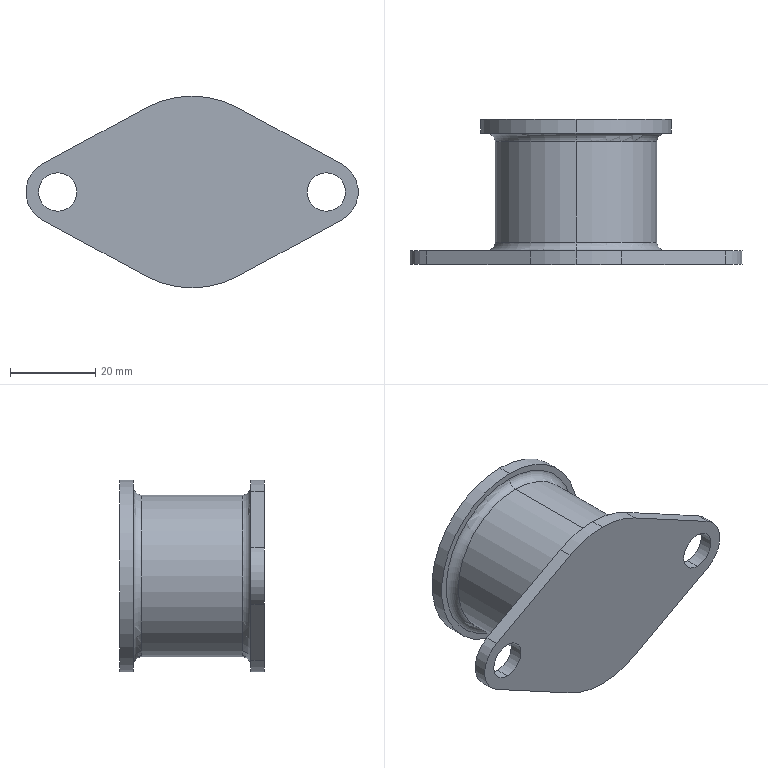Part | STEP file | SceondRB-45 | 1 solid | 29 faces | box 78 x 34 x 45 mm | volume 42765 mm3 | cylinder 15 | plane 8 | torus 4 | cone 2 | commonest cylinder face diameters 45 x5 9 x4 6.8 x2 15 x2 38 x2
STEP:
#1=CARTESIAN_POINT('',(0.,-19.75,-3.4));
#2=VERTEX_POINT('',#1);
#3=CARTESIAN_POINT('',(0.,-19.75,3.4));
#4=VERTEX_POINT('',#3);
#5=CARTESIAN_POINT('',(0.,-19.75,0.));
#6=DIRECTION('',(0.,1.,0.));
#7=DIRECTION('',(0.,0.,1.));
#8=AXIS2_PLACEMENT_3D('',#5,#6,#7);
#9=CIRCLE('',#8,3.4);
#10=EDGE_CURVE('',#2,#4,#9,.T.);
#11=ORIENTED_EDGE('',*,*,#10,.F.);
#12=CARTESIAN_POINT('',(0.,0.,-3.4));
#13=VERTEX_POINT('',#12);
#14=CARTESIAN_POINT('',(0.,0.,-3.4));
#15=DIRECTION('',(0.,1.,0.));
#16=VECTOR('',#15,1000.);
#17=LINE('',#14,#16);
#18=EDGE_CURVE('',#2,#13,#17,.T.);
#19=ORIENTED_EDGE('',*,*,#18,.T.);
#20=CARTESIAN_POINT('',(0.,0.,3.4));
#21=VERTEX_POINT('',#20);
#22=CARTESIAN_POINT('',(0.,0.,0.));
#23=DIRECTION('',(0.,1.,0.));
#24=DIRECTION('',(0.,0.,1.));
#25=AXIS2_PLACEMENT_3D('',#22,#23,#24);
#26=CIRCLE('',#25,3.4);
#27=EDGE_CURVE('',#13,#21,#26,.T.);
#28=ORIENTED_EDGE('',*,*,#27,.T.);
#29=CARTESIAN_POINT('',(0.,0.,3.4));
#30=DIRECTION('',(0.,1.,0.));
#31=VECTOR('',#30,1000.);
#32=LINE('',#29,#31);
#33=EDGE_CURVE('',#4,#21,#32,.T.);
#34=ORIENTED_EDGE('',*,*,#33,.F.);
#35=EDGE_LOOP('',(#11,#19,#28,#34));
#36=FACE_OUTER_BOUND('',#35,.T.);
#37=CARTESIAN_POINT('',(0.,0.,0.));
#38=DIRECTION('',(0.,1.,0.));
#39=DIRECTION('',(0.,0.,1.));
#40=AXIS2_PLACEMENT_3D('',#37,#38,#39);
#41=CYLINDRICAL_SURFACE('',#40,3.4);
#42=ADVANCED_FACE('',(#36),#41,.F.);
#43=CARTESIAN_POINT('',(0.,-21.793,0.));
#44=VERTEX_POINT('',#43);
#45=CARTESIAN_POINT('',(0.,-19.75,3.4));
#46=DIRECTION('',(0.,0.515,0.8572));
#47=VECTOR('',#46,1000.);
#48=LINE('',#45,#47);
#49=EDGE_CURVE('',#44,#4,#48,.T.);
#50=ORIENTED_EDGE('',*,*,#49,.F.);
#51=CARTESIAN_POINT('',(0.,-19.75,-3.4));
#52=DIRECTION('',(0.,0.515,-0.8572));
#53=VECTOR('',#52,1000.);
#54=LINE('',#51,#53);
#55=EDGE_CURVE('',#44,#2,#54,.T.);
#56=ORIENTED_EDGE('',*,*,#55,.T.);
#57=ORIENTED_EDGE('',*,*,#10,.T.);
#58=EDGE_LOOP('',(#50,#56,#57));
#59=FACE_OUTER_BOUND('',#58,.T.);
#60=CARTESIAN_POINT('',(0.,-19.75,0.));
#61=DIRECTION('',(0.,1.,0.));
#62=DIRECTION('',(0.,0.,1.));
#63=AXIS2_PLACEMENT_3D('',#60,#61,#62);
#64=CONICAL_SURFACE('',#63,3.4,1.03);
#65=ADVANCED_FACE('',(#59),#64,.F.);
#66=CARTESIAN_POINT('',(31.5,-34.,4.5));
#67=VERTEX_POINT('',#66);
#68=CARTESIAN_POINT('',(31.5,-34.,-4.5));
#69=VERTEX_POINT('',#68);
#70=CARTESIAN_POINT('',(31.5,-34.,0.));
#71=DIRECTION('',(0.,-1.,0.));
#72=DIRECTION('',(0.,0.,-1.));
#73=AXIS2_PLACEMENT_3D('',#70,#71,#72);
#74=CIRCLE('',#73,4.5);
#75=EDGE_CURVE('',#67,#69,#74,.T.);
#76=ORIENTED_EDGE('',*,*,#75,.T.);
#77=CARTESIAN_POINT('',(31.5,-30.8,-4.5));
#78=VERTEX_POINT('',#77);
#79=CARTESIAN_POINT('',(31.5,-34.,-4.5));
#80=DIRECTION('',(0.,1.,0.));
#81=VECTOR('',#80,1000.);
#82=LINE('',#79,#81);
#83=EDGE_CURVE('',#69,#78,#82,.T.);
#84=ORIENTED_EDGE('',*,*,#83,.T.);
#85=CARTESIAN_POINT('',(31.5,-30.8,4.5));
#86=VERTEX_POINT('',#85);
#87=CARTESIAN_POINT('',(31.5,-30.8,0.));
#88=DIRECTION('',(0.,-1.,0.));
#89=DIRECTION('',(0.,0.,-1.));
#90=AXIS2_PLACEMENT_3D('',#87,#88,#89);
#91=CIRCLE('',#90,4.5);
#92=EDGE_CURVE('',#86,#78,#91,.T.);
#93=ORIENTED_EDGE('',*,*,#92,.F.);
#94=CARTESIAN_POINT('',(31.5,-34.,4.5));
#95=DIRECTION('',(0.,1.,0.));
#96=VECTOR('',#95,1000.);
#97=LINE('',#94,#96);
#98=EDGE_CURVE('',#67,#86,#97,.T.);
#99=ORIENTED_EDGE('',*,*,#98,.F.);
#100=EDGE_LOOP('',(#76,#84,#93,#99));
#101=FACE_OUTER_BOUND('',#100,.T.);
#102=CARTESIAN_POINT('',(31.5,-34.,0.));
#103=DIRECTION('',(0.,1.,0.));
#104=DIRECTION('',(0.,0.,1.));
#105=AXIS2_PLACEMENT_3D('',#102,#103,#104);
#106=CYLINDRICAL_SURFACE('',#105,4.5);
#107=ADVANCED_FACE('',(#101),#106,.F.);
#108=CARTESIAN_POINT('',(-31.5,-34.,4.5));
#109=VERTEX_POINT('',#108);
#110=CARTESIAN_POINT('',(-31.5,-34.,-4.5));
#111=VERTEX_POINT('',#110);
#112=CARTESIAN_POINT('',(-31.5,-34.,0.));
#113=DIRECTION('',(0.,-1.,0.));
#114=DIRECTION('',(0.,0.,-1.));
#115=AXIS2_PLACEMENT_3D('',#112,#113,#114);
#116=CIRCLE('',#115,4.5);
#117=EDGE_CURVE('',#109,#111,#116,.T.);
#118=ORIENTED_EDGE('',*,*,#117,.T.);
#119=CARTESIAN_POINT('',(-31.5,-30.8,-4.5));
#120=VERTEX_POINT('',#119);
#121=CARTESIAN_POINT('',(-31.5,-34.,-4.5));
#122=DIRECTION('',(0.,1.,0.));
#123=VECTOR('',#122,1000.);
#124=LINE('',#121,#123);
#125=EDGE_CURVE('',#111,#120,#124,.T.);
#126=ORIENTED_EDGE('',*,*,#125,.T.);
#127=CARTESIAN_POINT('',(-31.5,-30.8,4.5));
#128=VERTEX_POINT('',#127);
#129=CARTESIAN_POINT('',(-31.5,-30.8,0.));
#130=DIRECTION('',(0.,-1.,0.));
#131=DIRECTION('',(0.,0.,-1.));
#132=AXIS2_PLACEMENT_3D('',#129,#130,#131);
#133=CIRCLE('',#132,4.5);
#134=EDGE_CURVE('',#128,#120,#133,.T.);
#135=ORIENTED_EDGE('',*,*,#134,.F.);
#136=CARTESIAN_POINT('',(-31.5,-34.,4.5));
#137=DIRECTION('',(0.,1.,0.));
#138=VECTOR('',#137,1000.);
#139=LINE('',#136,#138);
#140=EDGE_CURVE('',#109,#128,#139,.T.);
#141=ORIENTED_EDGE('',*,*,#140,.F.);
#142=EDGE_LOOP('',(#118,#126,#135,#141));
#143=FACE_OUTER_BOUND('',#142,.T.);
#144=CARTESIAN_POINT('',(-31.5,-34.,0.));
#145=DIRECTION('',(0.,1.,0.));
#146=DIRECTION('',(0.,0.,1.));
#147=AXIS2_PLACEMENT_3D('',#144,#145,#146);
#148=CYLINDRICAL_SURFACE('',#147,4.5);
#149=ADVANCED_FACE('',(#143),#148,.F.);
#150=CARTESIAN_POINT('',(0.,-34.,22.5));
#151=VERTEX_POINT('',#150);
#152=CARTESIAN_POINT('',(-10.714,-34.,19.785));
#153=VERTEX_POINT('',#152);
#154=CARTESIAN_POINT('',(0.,-34.,0.));
#155=DIRECTION('',(0.,-1.,0.));
#156=DIRECTION('',(0.,0.,-1.));
#157=AXIS2_PLACEMENT_3D('',#154,#155,#156);
#158=CIRCLE('',#157,22.5);
#159=EDGE_CURVE('',#151,#153,#158,.T.);
#160=ORIENTED_EDGE('',*,*,#159,.F.);
#161=CARTESIAN_POINT('',(0.,-30.8,22.5));
#162=VERTEX_POINT('',#161);
#163=CARTESIAN_POINT('',(0.,-34.,22.5));
#164=DIRECTION('',(0.,1.,0.));
#165=VECTOR('',#164,1000.);
#166=LINE('',#163,#165);
#167=EDGE_CURVE('',#151,#162,#166,.T.);
#168=ORIENTED_EDGE('',*,*,#167,.T.);
#169=CARTESIAN_POINT('',(-10.714,-30.8,19.785));
#170=VERTEX_POINT('',#169);
#171=CARTESIAN_POINT('',(0.,-30.8,0.));
#172=DIRECTION('',(0.,-1.,0.));
#173=DIRECTION('',(0.,0.,-1.));
#174=AXIS2_PLACEMENT_3D('',#171,#172,#173);
#175=CIRCLE('',#174,22.5);
#176=EDGE_CURVE('',#162,#170,#175,.T.);
#177=ORIENTED_EDGE('',*,*,#176,.T.);
#178=CARTESIAN_POINT('',(-10.714,-34.,19.785));
#179=DIRECTION('',(0.,1.,0.));
#180=VECTOR('',#179,1000.);
#181=LINE('',#178,#180);
#182=EDGE_CURVE('',#153,#170,#181,.T.);
#183=ORIENTED_EDGE('',*,*,#182,.F.);
#184=EDGE_LOOP('',(#160,#168,#177,#183));
#185=FACE_OUTER_BOUND('',#184,.T.);
#186=CARTESIAN_POINT('',(0.,-34.,0.));
#187=DIRECTION('',(0.,1.,0.));
#188=DIRECTION('',(0.,0.,1.));
#189=AXIS2_PLACEMENT_3D('',#186,#187,#188);
#190=CYLINDRICAL_SURFACE('',#189,22.5);
#191=ADVANCED_FACE('',(#185),#190,.T.);
#192=CARTESIAN_POINT('',(0.,-3.2,-21.));
#193=VERTEX_POINT('',#192);
#194=CARTESIAN_POINT('',(0.,-3.2,21.));
#195=VERTEX_POINT('',#194);
#196=CARTESIAN_POINT('',(0.,-3.2,0.));
#197=DIRECTION('',(0.,1.,0.));
#198=DIRECTION('',(0.,0.,1.));
#199=AXIS2_PLACEMENT_3D('',#196,#197,#198);
#200=CIRCLE('',#199,21.);
#201=EDGE_CURVE('',#193,#195,#200,.T.);
#202=ORIENTED_EDGE('',*,*,#201,.F.);
#203=CARTESIAN_POINT('',(0.,-5.2,-19.));
#204=VERTEX_POINT('',#203);
#205=CARTESIAN_POINT('',(0.,-5.2,-21.));
#206=DIRECTION('',(1.,0.,0.));
#207=DIRECTION('',(0.,0.,-1.));
#208=AXIS2_PLACEMENT_3D('',#205,#206,#207);
#209=CIRCLE('',#208,2.);
#210=EDGE_CURVE('',#193,#204,#209,.T.);
#211=ORIENTED_EDGE('',*,*,#210,.T.);
#212=CARTESIAN_POINT('',(0.,-5.2,19.));
#213=VERTEX_POINT('',#212);
#214=CARTESIAN_POINT('',(0.,-5.2,0.));
#215=DIRECTION('',(0.,1.,0.));
#216=DIRECTION('',(0.,0.,1.));
#217=AXIS2_PLACEMENT_3D('',#214,#215,#216);
#218=CIRCLE('',#217,19.);
#219=EDGE_CURVE('',#204,#213,#218,.T.);
#220=ORIENTED_EDGE('',*,*,#219,.T.);
#221=CARTESIAN_POINT('',(0.,-5.2,21.));
#222=DIRECTION('',(-1.,0.,0.));
#223=DIRECTION('',(0.,0.,1.));
#224=AXIS2_PLACEMENT_3D('',#221,#222,#223);
#225=CIRCLE('',#224,2.);
#226=EDGE_CURVE('',#195,#213,#225,.T.);
#227=ORIENTED_EDGE('',*,*,#226,.F.);
#228=EDGE_LOOP('',(#202,#211,#220,#227));
#229=FACE_OUTER_BOUND('',#228,.T.);
#230=CARTESIAN_POINT('',(0.,-5.2,0.));
#231=DIRECTION('',(0.,1.,0.));
#232=DIRECTION('',(0.,0.,1.));
#233=AXIS2_PLACEMENT_3D('',#230,#231,#232);
#234=TOROIDAL_SURFACE('',#233,21.,2.);
#235=ADVANCED_FACE('',(#229),#234,.F.);
#236=CARTESIAN_POINT('',(0.,-28.8,19.));
#237=VERTEX_POINT('',#236);
#238=CARTESIAN_POINT('',(0.,-28.8,-19.));
#239=VERTEX_POINT('',#238);
#240=CARTESIAN_POINT('',(0.,-28.8,0.));
#241=DIRECTION('',(0.,1.,0.));
#242=DIRECTION('',(0.,0.,1.));
#243=AXIS2_PLACEMENT_3D('',#240,#241,#242);
#244=CIRCLE('',#243,19.);
#245=EDGE_CURVE('',#237,#239,#244,.T.);
#246=ORIENTED_EDGE('',*,*,#245,.T.);
#247=CARTESIAN_POINT('',(0.,0.,-19.));
#248=DIRECTION('',(0.,1.,0.));
#249=VECTOR('',#248,1000.);
#250=LINE('',#247,#249);
#251=EDGE_CURVE('',#239,#204,#250,.T.);
#252=ORIENTED_EDGE('',*,*,#251,.T.);
#253=CARTESIAN_POINT('',(0.,-5.2,0.));
#254=DIRECTION('',(0.,1.,0.));
#255=DIRECTION('',(0.,0.,1.));
#256=AXIS2_PLACEMENT_3D('',#253,#254,#255);
#257=CIRCLE('',#256,19.);
#258=EDGE_CURVE('',#213,#204,#257,.T.);
#259=ORIENTED_EDGE('',*,*,#258,.F.);
#260=CARTESIAN_POINT('',(0.,0.,19.));
#261=DIRECTION('',(0.,1.,0.));
#262=VECTOR('',#261,1000.);
#263=LINE('',#260,#262);
#264=EDGE_CURVE('',#237,#213,#263,.T.);
#265=ORIENTED_EDGE('',*,*,#264,.F.);
#266=EDGE_LOOP('',(#246,#252,#259,#265));
#267=FACE_OUTER_BOUND('',#266,.T.);
#268=CARTESIAN_POINT('',(0.,0.,0.));
#269=DIRECTION('',(0.,1.,0.));
#270=DIRECTION('',(0.,0.,1.));
#271=AXIS2_PLACEMENT_3D('',#268,#269,#270);
#272=CYLINDRICAL_SURFACE('',#271,19.);
#273=ADVANCED_FACE('',(#267),#272,.T.);
#274=CARTESIAN_POINT('',(0.,-28.8,0.));
#275=DIRECTION('',(0.,1.,0.));
#276=DIRECTION('',(0.,0.,1.));
#277=AXIS2_PLACEMENT_3D('',#274,#275,#276);
#278=CIRCLE('',#277,19.);
#279=EDGE_CURVE('',#239,#237,#278,.T.);
#280=ORIENTED_EDGE('',*,*,#279,.F.);
#281=CARTESIAN_POINT('',(0.,-30.8,-21.));
#282=VERTEX_POINT('',#281);
#283=CARTESIAN_POINT('',(0.,-28.8,-21.));
#284=DIRECTION('',(1.,0.,0.));
#285=DIRECTION('',(0.,0.,-1.));
#286=AXIS2_PLACEMENT_3D('',#283,#284,#285);
#287=CIRCLE('',#286,2.);
#288=EDGE_CURVE('',#239,#282,#287,.T.);
#289=ORIENTED_EDGE('',*,*,#288,.T.);
#290=CARTESIAN_POINT('',(0.,-30.8,21.));
#291=VERTEX_POINT('',#290);
#292=CARTESIAN_POINT('',(0.,-30.8,0.));
#293=DIRECTION('',(0.,-1.,0.));
#294=DIRECTION('',(0.,0.,1.));
#295=AXIS2_PLACEMENT_3D('',#292,#293,#294);
#296=CIRCLE('',#295,21.);
#297=EDGE_CURVE('',#291,#282,#296,.T.);
#298=ORIENTED_EDGE('',*,*,#297,.F.);
#299=CARTESIAN_POINT('',(0.,-28.8,21.));
#300=DIRECTION('',(-1.,0.,0.));
#301=DIRECTION('',(0.,0.,1.));
#302=AXIS2_PLACEMENT_3D('',#299,#300,#301);
#303=CIRCLE('',#302,2.);
#304=EDGE_CURVE('',#237,#291,#303,.T.);
#305=ORIENTED_EDGE('',*,*,#304,.F.);
#306=EDGE_LOOP('',(#280,#289,#298,#305));
#307=FACE_OUTER_BOUND('',#306,.T.);
#308=CARTESIAN_POINT('',(0.,-28.8,0.));
#309=DIRECTION('',(0.,1.,0.));
#310=DIRECTION('',(0.,0.,1.));
#311=AXIS2_PLACEMENT_3D('',#308,#309,#310);
#312=TOROIDAL_SURFACE('',#311,21.,2.);
#313=ADVANCED_FACE('',(#307),#312,.F.);
#314=CARTESIAN_POINT('',(0.,-3.2,22.5));
#315=VERTEX_POINT('',#314);
#316=CARTESIAN_POINT('',(0.,-3.2,-22.5));
#317=VERTEX_POINT('',#316);
#318=CARTESIAN_POINT('',(0.,-3.2,0.));
#319=DIRECTION('',(0.,1.,0.));
#320=DIRECTION('',(0.,0.,1.));
#321=AXIS2_PLACEMENT_3D('',#318,#319,#320);
#322=CIRCLE('',#321,22.5);
#323=EDGE_CURVE('',#315,#317,#322,.T.);
#324=ORIENTED_EDGE('',*,*,#323,.T.);
#325=CARTESIAN_POINT('',(0.,0.,-22.5));
#326=VERTEX_POINT('',#325);
#327=CARTESIAN_POINT('',(0.,0.,-22.5));
#328=DIRECTION('',(0.,1.,0.));
#329=VECTOR('',#328,1000.);
#330=LINE('',#327,#329);
#331=EDGE_CURVE('',#317,#326,#330,.T.);
#332=ORIENTED_EDGE('',*,*,#331,.T.);
#333=CARTESIAN_POINT('',(0.,0.,22.5));
#334=VERTEX_POINT('',#333);
#335=CARTESIAN_POINT('',(0.,0.,0.));
#336=DIRECTION('',(0.,1.,0.));
#337=DIRECTION('',(0.,0.,1.));
#338=AXIS2_PLACEMENT_3D('',#335,#336,#337);
#339=CIRCLE('',#338,22.5);
#340=EDGE_CURVE('',#334,#326,#339,.T.);
#341=ORIENTED_EDGE('',*,*,#340,.F.);
#342=CARTESIAN_POINT('',(0.,0.,22.5));
#343=DIRECTION('',(0.,1.,0.));
#344=VECTOR('',#343,1000.);
#345=LINE('',#342,#344);
#346=EDGE_CURVE('',#315,#334,#345,.T.);
#347=ORIENTED_EDGE('',*,*,#346,.F.);
#348=EDGE_LOOP('',(#324,#332,#341,#347));
#349=FACE_OUTER_BOUND('',#348,.T.);
#350=CARTESIAN_POINT('',(0.,0.,0.));
#351=DIRECTION('',(0.,1.,0.));
#352=DIRECTION('',(0.,0.,1.));
#353=AXIS2_PLACEMENT_3D('',#350,#351,#352);
#354=CYLINDRICAL_SURFACE('',#353,22.5);
#355=ADVANCED_FACE('',(#349),#354,.T.);
#356=ORIENTED_EDGE('',*,*,#331,.F.);
#357=CARTESIAN_POINT('',(0.,-3.2,0.));
#358=DIRECTION('',(0.,1.,0.));
#359=DIRECTION('',(0.,0.,1.));
#360=AXIS2_PLACEMENT_3D('',#357,#358,#359);
#361=CIRCLE('',#360,22.5);
#362=EDGE_CURVE('',#317,#315,#361,.T.);
#363=ORIENTED_EDGE('',*,*,#362,.T.);
#364=ORIENTED_EDGE('',*,*,#346,.T.);
#365=CARTESIAN_POINT('',(0.,0.,0.));
#366=DIRECTION('',(0.,1.,0.));
#367=DIRECTION('',(0.,0.,1.));
#368=AXIS2_PLACEMENT_3D('',#365,#366,#367);
#369=CIRCLE('',#368,22.5);
#370=EDGE_CURVE('',#326,#334,#369,.T.);
#371=ORIENTED_EDGE('',*,*,#370,.F.);
#372=EDGE_LOOP('',(#356,#363,#364,#371));
#373=FACE_OUTER_BOUND('',#372,.T.);
#374=CARTESIAN_POINT('',(0.,0.,0.));
#375=DIRECTION('',(0.,1.,0.));
#376=DIRECTION('',(0.,0.,1.));
#377=AXIS2_PLACEMENT_3D('',#374,#375,#376);
#378=CYLINDRICAL_SURFACE('',#377,22.5);
#379=ADVANCED_FACE('',(#373),#378,.T.);
#380=CARTESIAN_POINT('',(0.,0.,0.));
#381=DIRECTION('',(0.,1.,0.));
#382=DIRECTION('',(0.,0.,1.));
#383=AXIS2_PLACEMENT_3D('',#380,#381,#382);
#384=CIRCLE('',#383,3.4);
#385=EDGE_CURVE('',#21,#13,#384,.T.);
#386=ORIENTED_EDGE('',*,*,#385,.F.);
#387=ORIENTED_EDGE('',*,*,#27,.F.);
#388=EDGE_LOOP('',(#386,#387));
#389=FACE_BOUND('',#388,.T.);
#390=ORIENTED_EDGE('',*,*,#340,.T.);
#391=ORIENTED_EDGE('',*,*,#370,.T.);
#392=EDGE_LOOP('',(#390,#391));
#393=FACE_OUTER_BOUND('',#392,.T.);
#394=CARTESIAN_POINT('',(22.5,0.,0.));
#395=DIRECTION('',(0.,-1.,0.));
#396=DIRECTION('',(0.,0.,-1.));
#397=AXIS2_PLACEMENT_3D('',#394,#395,#396);
#398=PLANE('',#397);
#399=ADVANCED_FACE('',(#389,#393),#398,.F.);
#400=ORIENTED_EDGE('',*,*,#288,.F.);
#401=ORIENTED_EDGE('',*,*,#245,.F.);
#402=ORIENTED_EDGE('',*,*,#304,.T.);
#403=CARTESIAN_POINT('',(0.,-30.8,0.));
#404=DIRECTION('',(0.,-1.,0.));
#405=DIRECTION('',(0.,0.,1.));
#406=AXIS2_PLACEMENT_3D('',#403,#404,#405);
#407=CIRCLE('',#406,21.);
#408=EDGE_CURVE('',#282,#291,#407,.T.);
#409=ORIENTED_EDGE('',*,*,#408,.F.);
#410=EDGE_LOOP('',(#400,#401,#402,#409));
#411=FACE_OUTER_BOUND('',#410,.T.);
#412=CARTESIAN_POINT('',(0.,-28.8,0.));
#413=DIRECTION('',(0.,1.,0.));
#414=DIRECTION('',(0.,0.,1.));
#415=AXIS2_PLACEMENT_3D('',#412,#413,#414);
#416=TOROIDAL_SURFACE('',#415,21.,2.);
#417=ADVANCED_FACE('',(#411),#416,.F.);
#418=ORIENTED_EDGE('',*,*,#251,.F.);
#419=ORIENTED_EDGE('',*,*,#279,.T.);
#420=ORIENTED_EDGE('',*,*,#264,.T.);
#421=ORIENTED_EDGE('',*,*,#219,.F.);
#422=EDGE_LOOP('',(#418,#419,#420,#421));
#423=FACE_OUTER_BOUND('',#422,.T.);
#424=CARTESIAN_POINT('',(0.,0.,0.));
#425=DIRECTION('',(0.,1.,0.));
#426=DIRECTION('',(0.,0.,1.));
#427=AXIS2_PLACEMENT_3D('',#424,#425,#426);
#428=CYLINDRICAL_SURFACE('',#427,19.);
#429=ADVANCED_FACE('',(#423),#428,.T.);
#430=ORIENTED_EDGE('',*,*,#210,.F.);
#431=CARTESIAN_POINT('',(0.,-3.2,0.));
#432=DIRECTION('',(0.,1.,0.));
#433=DIRECTION('',(0.,0.,1.));
#434=AXIS2_PLACEMENT_3D('',#431,#432,#433);
#435=CIRCLE('',#434,21.);
#436=EDGE_CURVE('',#195,#193,#435,.T.);
#437=ORIENTED_EDGE('',*,*,#436,.F.);
#438=ORIENTED_EDGE('',*,*,#226,.T.);
#439=ORIENTED_EDGE('',*,*,#258,.T.);
#440=EDGE_LOOP('',(#430,#437,#438,#439));
#441=FACE_OUTER_BOUND('',#440,.T.);
#442=CARTESIAN_POINT('',(0.,-5.2,0.));
#443=DIRECTION('',(0.,1.,0.));
#444=DIRECTION('',(0.,0.,1.));
#445=AXIS2_PLACEMENT_3D('',#442,#443,#444);
#446=TOROIDAL_SURFACE('',#445,21.,2.);
#447=ADVANCED_FACE('',(#441),#446,.F.);
#448=ORIENTED_EDGE('',*,*,#323,.F.);
#449=ORIENTED_EDGE('',*,*,#362,.F.);
#450=EDGE_LOOP('',(#448,#449));
#451=FACE_OUTER_BOUND('',#450,.T.);
#452=ORIENTED_EDGE('',*,*,#436,.T.);
#453=ORIENTED_EDGE('',*,*,#201,.T.);
#454=EDGE_LOOP('',(#452,#453));
#455=FACE_BOUND('',#454,.T.);
#456=CARTESIAN_POINT('',(21.,-3.2,0.));
#457=DIRECTION('',(0.,1.,0.));
#458=DIRECTION('',(0.,0.,1.));
#459=AXIS2_PLACEMENT_3D('',#456,#457,#458);
#460=PLANE('',#459);
#461=ADVANCED_FACE('',(#451,#455),#460,.F.);
#462=ORIENTED_EDGE('',*,*,#92,.T.);
#463=CARTESIAN_POINT('',(31.5,-30.8,0.));
#464=DIRECTION('',(0.,-1.,0.));
#465=DIRECTION('',(0.,0.,-1.));
#466=AXIS2_PLACEMENT_3D('',#463,#464,#465);
#467=CIRCLE('',#466,4.5);
#468=EDGE_CURVE('',#78,#86,#467,.T.);
#469=ORIENTED_EDGE('',*,*,#468,.T.);
#470=EDGE_LOOP('',(#462,#469));
#471=FACE_BOUND('',#470,.T.);
#472=CARTESIAN_POINT('',(-35.071,-30.8,6.595));
#473=VERTEX_POINT('',#472);
#474=CARTESIAN_POINT('',(-35.071,-30.8,-6.595));
#475=VERTEX_POINT('',#474);
#476=CARTESIAN_POINT('',(-31.5,-30.8,0.));
#477=DIRECTION('',(0.,-1.,0.));
#478=DIRECTION('',(0.,0.,-1.));
#479=AXIS2_PLACEMENT_3D('',#476,#477,#478);
#480=CIRCLE('',#479,7.5);
#481=EDGE_CURVE('',#473,#475,#480,.T.);
#482=ORIENTED_EDGE('',*,*,#481,.F.);
#483=CARTESIAN_POINT('',(-35.071,-30.8,6.595));
#484=DIRECTION('',(-0.8793,0.,-0.4762));
#485=VECTOR('',#484,1000.);
#486=LINE('',#483,#485);
#487=EDGE_CURVE('',#170,#473,#486,.T.);
#488=ORIENTED_EDGE('',*,*,#487,.F.);
#489=ORIENTED_EDGE('',*,*,#176,.F.);
#490=CARTESIAN_POINT('',(10.714,-30.8,19.785));
#491=VERTEX_POINT('',#490);
#492=CARTESIAN_POINT('',(0.,-30.8,0.));
#493=DIRECTION('',(0.,-1.,0.));
#494=DIRECTION('',(0.,0.,-1.));
#495=AXIS2_PLACEMENT_3D('',#492,#493,#494);
#496=CIRCLE('',#495,22.5);
#497=EDGE_CURVE('',#491,#162,#496,.T.);
#498=ORIENTED_EDGE('',*,*,#497,.F.);
#499=CARTESIAN_POINT('',(35.071,-30.8,6.595));
#500=VERTEX_POINT('',#499);
#501=CARTESIAN_POINT('',(10.714,-30.8,19.785));
#502=DIRECTION('',(-0.8793,0.,0.4762));
#503=VECTOR('',#502,1000.);
#504=LINE('',#501,#503);
#505=EDGE_CURVE('',#500,#491,#504,.T.);
#506=ORIENTED_EDGE('',*,*,#505,.F.);
#507=CARTESIAN_POINT('',(35.071,-30.8,-6.595));
#508=VERTEX_POINT('',#507);
#509=CARTESIAN_POINT('',(31.5,-30.8,0.));
#510=DIRECTION('',(0.,-1.,0.));
#511=DIRECTION('',(0.,0.,-1.));
#512=AXIS2_PLACEMENT_3D('',#509,#510,#511);
#513=CIRCLE('',#512,7.5);
#514=EDGE_CURVE('',#508,#500,#513,.T.);
#515=ORIENTED_EDGE('',*,*,#514,.F.);
#516=CARTESIAN_POINT('',(10.714,-30.8,-19.785));
#517=VERTEX_POINT('',#516);
#518=CARTESIAN_POINT('',(10.714,-30.8,-19.785));
#519=DIRECTION('',(0.8793,0.,0.4762));
#520=VECTOR('',#519,1000.);
#521=LINE('',#518,#520);
#522=EDGE_CURVE('',#517,#508,#521,.T.);
#523=ORIENTED_EDGE('',*,*,#522,.F.);
#524=CARTESIAN_POINT('',(-10.714,-30.8,-19.785));
#525=VERTEX_POINT('',#524);
#526=CARTESIAN_POINT('',(0.,-30.8,0.));
#527=DIRECTION('',(0.,-1.,0.));
#528=DIRECTION('',(0.,0.,-1.));
#529=AXIS2_PLACEMENT_3D('',#526,#527,#528);
#530=CIRCLE('',#529,22.5);
#531=EDGE_CURVE('',#525,#517,#530,.T.);
#532=ORIENTED_EDGE('',*,*,#531,.F.);
#533=CARTESIAN_POINT('',(-35.071,-30.8,-6.595));
#534=DIRECTION('',(0.8793,0.,-0.4762));
#535=VECTOR('',#534,1000.);
#536=LINE('',#533,#535);
#537=EDGE_CURVE('',#475,#525,#536,.T.);
#538=ORIENTED_EDGE('',*,*,#537,.F.);
#539=EDGE_LOOP('',(#482,#488,#489,#498,#506,#515,#523,#532,#538));
#540=FACE_OUTER_BOUND('',#539,.T.);
#541=ORIENTED_EDGE('',*,*,#134,.T.);
#542=CARTESIAN_POINT('',(-31.5,-30.8,0.));
#543=DIRECTION('',(0.,-1.,0.));
#544=DIRECTION('',(0.,0.,-1.));
#545=AXIS2_PLACEMENT_3D('',#542,#543,#544);
#546=CIRCLE('',#545,4.5);
#547=EDGE_CURVE('',#120,#128,#546,.T.);
#548=ORIENTED_EDGE('',*,*,#547,.T.);
#549=EDGE_LOOP('',(#541,#548));
#550=FACE_BOUND('',#549,.T.);
#551=ORIENTED_EDGE('',*,*,#297,.T.);
#552=ORIENTED_EDGE('',*,*,#408,.T.);
#553=EDGE_LOOP('',(#551,#552));
#554=FACE_BOUND('',#553,.T.);
#555=CARTESIAN_POINT('',(-31.5,-30.8,0.));
#556=DIRECTION('',(0.,-1.,0.));
#557=DIRECTION('',(0.,0.,-1.));
#558=AXIS2_PLACEMENT_3D('',#555,#556,#557);
#559=PLANE('',#558);
#560=ADVANCED_FACE('',(#471,#540,#550,#554),#559,.F.);
#561=ORIENTED_EDGE('',*,*,#117,.F.);
#562=CARTESIAN_POINT('',(-31.5,-34.,0.));
#563=DIRECTION('',(0.,-1.,0.));
#564=DIRECTION('',(0.,0.,-1.));
#565=AXIS2_PLACEMENT_3D('',#562,#563,#564);
#566=CIRCLE('',#565,4.5);
#567=EDGE_CURVE('',#111,#109,#566,.T.);
#568=ORIENTED_EDGE('',*,*,#567,.F.);
#569=EDGE_LOOP('',(#561,#568));
#570=FACE_BOUND('',#569,.T.);
#571=CARTESIAN_POINT('',(-35.071,-34.,6.595));
#572=VERTEX_POINT('',#571);
#573=CARTESIAN_POINT('',(-35.071,-34.,-6.595));
#574=VERTEX_POINT('',#573);
#575=CARTESIAN_POINT('',(-31.5,-34.,0.));
#576=DIRECTION('',(0.,-1.,0.));
#577=DIRECTION('',(0.,0.,-1.));
#578=AXIS2_PLACEMENT_3D('',#575,#576,#577);
#579=CIRCLE('',#578,7.5);
#580=EDGE_CURVE('',#572,#574,#579,.T.);
#581=ORIENTED_EDGE('',*,*,#580,.T.);
#582=CARTESIAN_POINT('',(-10.714,-34.,-19.785));
#583=VERTEX_POINT('',#582);
#584=CARTESIAN_POINT('',(-35.071,-34.,-6.595));
#585=DIRECTION('',(0.8793,0.,-0.4762));
#586=VECTOR('',#585,1000.);
#587=LINE('',#584,#586);
#588=EDGE_CURVE('',#574,#583,#587,.T.);
#589=ORIENTED_EDGE('',*,*,#588,.T.);
#590=CARTESIAN_POINT('',(10.714,-34.,-19.785));
#591=VERTEX_POINT('',#590);
#592=CARTESIAN_POINT('',(0.,-34.,0.));
#593=DIRECTION('',(0.,-1.,0.));
#594=DIRECTION('',(0.,0.,-1.));
#595=AXIS2_PLACEMENT_3D('',#592,#593,#594);
#596=CIRCLE('',#595,22.5);
#597=EDGE_CURVE('',#583,#591,#596,.T.);
#598=ORIENTED_EDGE('',*,*,#597,.T.);
#599=CARTESIAN_POINT('',(35.071,-34.,-6.595));
#600=VERTEX_POINT('',#599);
#601=CARTESIAN_POINT('',(10.714,-34.,-19.785));
#602=DIRECTION('',(0.8793,0.,0.4762));
#603=VECTOR('',#602,1000.);
#604=LINE('',#601,#603);
#605=EDGE_CURVE('',#591,#600,#604,.T.);
#606=ORIENTED_EDGE('',*,*,#605,.T.);
#607=CARTESIAN_POINT('',(35.071,-34.,6.595));
#608=VERTEX_POINT('',#607);
#609=CARTESIAN_POINT('',(31.5,-34.,0.));
#610=DIRECTION('',(0.,-1.,0.));
#611=DIRECTION('',(0.,0.,-1.));
#612=AXIS2_PLACEMENT_3D('',#609,#610,#611);
#613=CIRCLE('',#612,7.5);
#614=EDGE_CURVE('',#600,#608,#613,.T.);
#615=ORIENTED_EDGE('',*,*,#614,.T.);
#616=CARTESIAN_POINT('',(10.714,-34.,19.785));
#617=VERTEX_POINT('',#616);
#618=CARTESIAN_POINT('',(10.714,-34.,19.785));
#619=DIRECTION('',(-0.8793,0.,0.4762));
#620=VECTOR('',#619,1000.);
#621=LINE('',#618,#620);
#622=EDGE_CURVE('',#608,#617,#621,.T.);
#623=ORIENTED_EDGE('',*,*,#622,.T.);
#624=CARTESIAN_POINT('',(0.,-34.,0.));
#625=DIRECTION('',(0.,-1.,0.));
#626=DIRECTION('',(0.,0.,-1.));
#627=AXIS2_PLACEMENT_3D('',#624,#625,#626);
#628=CIRCLE('',#627,22.5);
#629=EDGE_CURVE('',#617,#151,#628,.T.);
#630=ORIENTED_EDGE('',*,*,#629,.T.);
#631=ORIENTED_EDGE('',*,*,#159,.T.);
#632=CARTESIAN_POINT('',(-35.071,-34.,6.595));
#633=DIRECTION('',(-0.8793,0.,-0.4762));
#634=VECTOR('',#633,1000.);
#635=LINE('',#632,#634);
#636=EDGE_CURVE('',#153,#572,#635,.T.);
#637=ORIENTED_EDGE('',*,*,#636,.T.);
#638=EDGE_LOOP('',(#581,#589,#598,#606,#615,#623,#630,#631,#637));
#639=FACE_OUTER_BOUND('',#638,.T.);
#640=ORIENTED_EDGE('',*,*,#75,.F.);
#641=CARTESIAN_POINT('',(31.5,-34.,0.));
#642=DIRECTION('',(0.,-1.,0.));
#643=DIRECTION('',(0.,0.,-1.));
#644=AXIS2_PLACEMENT_3D('',#641,#642,#643);
#645=CIRCLE('',#644,4.5);
#646=EDGE_CURVE('',#69,#67,#645,.T.);
#647=ORIENTED_EDGE('',*,*,#646,.F.);
#648=EDGE_LOOP('',(#640,#647));
#649=FACE_BOUND('',#648,.T.);
#650=CARTESIAN_POINT('',(-31.5,-34.,0.));
#651=DIRECTION('',(0.,-1.,0.));
#652=DIRECTION('',(0.,0.,-1.));
#653=AXIS2_PLACEMENT_3D('',#650,#651,#652);
#654=PLANE('',#653);
#655=ADVANCED_FACE('',(#570,#639,#649),#654,.T.);
#656=ORIENTED_EDGE('',*,*,#481,.T.);
#657=CARTESIAN_POINT('',(-35.071,-34.,-6.595));
#658=DIRECTION('',(0.,1.,0.));
#659=VECTOR('',#658,1000.);
#660=LINE('',#657,#659);
#661=EDGE_CURVE('',#574,#475,#660,.T.);
#662=ORIENTED_EDGE('',*,*,#661,.F.);
#663=ORIENTED_EDGE('',*,*,#580,.F.);
#664=CARTESIAN_POINT('',(-35.071,-34.,6.595));
#665=DIRECTION('',(0.,1.,0.));
#666=VECTOR('',#665,1000.);
#667=LINE('',#664,#666);
#668=EDGE_CURVE('',#572,#473,#667,.T.);
#669=ORIENTED_EDGE('',*,*,#668,.T.);
#670=EDGE_LOOP('',(#656,#662,#663,#669));
#671=FACE_OUTER_BOUND('',#670,.T.);
#672=CARTESIAN_POINT('',(-31.5,-34.,0.));
#673=DIRECTION('',(0.,1.,0.));
#674=DIRECTION('',(0.,0.,1.));
#675=AXIS2_PLACEMENT_3D('',#672,#673,#674);
#676=CYLINDRICAL_SURFACE('',#675,7.5);
#677=ADVANCED_FACE('',(#671),#676,.T.);
#678=ORIENTED_EDGE('',*,*,#537,.T.);
#679=CARTESIAN_POINT('',(-10.714,-34.,-19.785));
#680=DIRECTION('',(0.,1.,0.));
#681=VECTOR('',#680,1000.);
#682=LINE('',#679,#681);
#683=EDGE_CURVE('',#583,#525,#682,.T.);
#684=ORIENTED_EDGE('',*,*,#683,.F.);
#685=ORIENTED_EDGE('',*,*,#588,.F.);
#686=ORIENTED_EDGE('',*,*,#661,.T.);
#687=EDGE_LOOP('',(#678,#684,#685,#686));
#688=FACE_OUTER_BOUND('',#687,.T.);
#689=CARTESIAN_POINT('',(-35.071,-34.,-6.595));
#690=DIRECTION('',(0.4762,0.,0.8793));
#691=DIRECTION('',(0.8793,0.,-0.4762));
#692=AXIS2_PLACEMENT_3D('',#689,#690,#691);
#693=PLANE('',#692);
#694=ADVANCED_FACE('',(#688),#693,.F.);
#695=ORIENTED_EDGE('',*,*,#531,.T.);
#696=CARTESIAN_POINT('',(10.714,-34.,-19.785));
#697=DIRECTION('',(0.,1.,0.));
#698=VECTOR('',#697,1000.);
#699=LINE('',#696,#698);
#700=EDGE_CURVE('',#591,#517,#699,.T.);
#701=ORIENTED_EDGE('',*,*,#700,.F.);
#702=ORIENTED_EDGE('',*,*,#597,.F.);
#703=ORIENTED_EDGE('',*,*,#683,.T.);
#704=EDGE_LOOP('',(#695,#701,#702,#703));
#705=FACE_OUTER_BOUND('',#704,.T.);
#706=CARTESIAN_POINT('',(0.,-34.,0.));
#707=DIRECTION('',(0.,1.,0.));
#708=DIRECTION('',(0.,0.,1.));
#709=AXIS2_PLACEMENT_3D('',#706,#707,#708);
#710=CYLINDRICAL_SURFACE('',#709,22.5);
#711=ADVANCED_FACE('',(#705),#710,.T.);
#712=ORIENTED_EDGE('',*,*,#522,.T.);
#713=CARTESIAN_POINT('',(35.071,-34.,-6.595));
#714=DIRECTION('',(0.,1.,0.));
#715=VECTOR('',#714,1000.);
#716=LINE('',#713,#715);
#717=EDGE_CURVE('',#600,#508,#716,.T.);
#718=ORIENTED_EDGE('',*,*,#717,.F.);
#719=ORIENTED_EDGE('',*,*,#605,.F.);
#720=ORIENTED_EDGE('',*,*,#700,.T.);
#721=EDGE_LOOP('',(#712,#718,#719,#720));
#722=FACE_OUTER_BOUND('',#721,.T.);
#723=CARTESIAN_POINT('',(10.714,-34.,-19.785));
#724=DIRECTION('',(-0.4762,0.,0.8793));
#725=DIRECTION('',(0.8793,0.,0.4762));
#726=AXIS2_PLACEMENT_3D('',#723,#724,#725);
#727=PLANE('',#726);
#728=ADVANCED_FACE('',(#722),#727,.F.);
#729=ORIENTED_EDGE('',*,*,#514,.T.);
#730=CARTESIAN_POINT('',(35.071,-34.,6.595));
#731=DIRECTION('',(0.,1.,0.));
#732=VECTOR('',#731,1000.);
#733=LINE('',#730,#732);
#734=EDGE_CURVE('',#608,#500,#733,.T.);
#735=ORIENTED_EDGE('',*,*,#734,.F.);
#736=ORIENTED_EDGE('',*,*,#614,.F.);
#737=ORIENTED_EDGE('',*,*,#717,.T.);
#738=EDGE_LOOP('',(#729,#735,#736,#737));
#739=FACE_OUTER_BOUND('',#738,.T.);
#740=CARTESIAN_POINT('',(31.5,-34.,0.));
#741=DIRECTION('',(0.,1.,0.));
#742=DIRECTION('',(0.,0.,1.));
#743=AXIS2_PLACEMENT_3D('',#740,#741,#742);
#744=CYLINDRICAL_SURFACE('',#743,7.5);
#745=ADVANCED_FACE('',(#739),#744,.T.);
#746=ORIENTED_EDGE('',*,*,#505,.T.);
#747=CARTESIAN_POINT('',(10.714,-34.,19.785));
#748=DIRECTION('',(0.,1.,0.));
#749=VECTOR('',#748,1000.);
#750=LINE('',#747,#749);
#751=EDGE_CURVE('',#617,#491,#750,.T.);
#752=ORIENTED_EDGE('',*,*,#751,.F.);
#753=ORIENTED_EDGE('',*,*,#622,.F.);
#754=ORIENTED_EDGE('',*,*,#734,.T.);
#755=EDGE_LOOP('',(#746,#752,#753,#754));
#756=FACE_OUTER_BOUND('',#755,.T.);
#757=CARTESIAN_POINT('',(10.714,-34.,19.785));
#758=DIRECTION('',(-0.4762,0.,-0.8793));
#759=DIRECTION('',(-0.8793,0.,0.4762));
#760=AXIS2_PLACEMENT_3D('',#757,#758,#759);
#761=PLANE('',#760);
#762=ADVANCED_FACE('',(#756),#761,.F.);
#763=ORIENTED_EDGE('',*,*,#167,.F.);
#764=ORIENTED_EDGE('',*,*,#629,.F.);
#765=ORIENTED_EDGE('',*,*,#751,.T.);
#766=ORIENTED_EDGE('',*,*,#497,.T.);
#767=EDGE_LOOP('',(#763,#764,#765,#766));
#768=FACE_OUTER_BOUND('',#767,.T.);
#769=CARTESIAN_POINT('',(0.,-34.,0.));
#770=DIRECTION('',(0.,1.,0.));
#771=DIRECTION('',(0.,0.,1.));
#772=AXIS2_PLACEMENT_3D('',#769,#770,#771);
#773=CYLINDRICAL_SURFACE('',#772,22.5);
#774=ADVANCED_FACE('',(#768),#773,.T.);
#775=ORIENTED_EDGE('',*,*,#487,.T.);
#776=ORIENTED_EDGE('',*,*,#668,.F.);
#777=ORIENTED_EDGE('',*,*,#636,.F.);
#778=ORIENTED_EDGE('',*,*,#182,.T.);
#779=EDGE_LOOP('',(#775,#776,#777,#778));
#780=FACE_OUTER_BOUND('',#779,.T.);
#781=CARTESIAN_POINT('',(-35.071,-34.,6.595));
#782=DIRECTION('',(0.4762,0.,-0.8793));
#783=DIRECTION('',(-0.8793,0.,-0.4762));
#784=AXIS2_PLACEMENT_3D('',#781,#782,#783);
#785=PLANE('',#784);
#786=ADVANCED_FACE('',(#780),#785,.F.);
#787=ORIENTED_EDGE('',*,*,#125,.F.);
#788=ORIENTED_EDGE('',*,*,#567,.T.);
#789=ORIENTED_EDGE('',*,*,#140,.T.);
#790=ORIENTED_EDGE('',*,*,#547,.F.);
#791=EDGE_LOOP('',(#787,#788,#789,#790));
#792=FACE_OUTER_BOUND('',#791,.T.);
#793=CARTESIAN_POINT('',(-31.5,-34.,0.));
#794=DIRECTION('',(0.,1.,0.));
#795=DIRECTION('',(0.,0.,1.));
#796=AXIS2_PLACEMENT_3D('',#793,#794,#795);
#797=CYLINDRICAL_SURFACE('',#796,4.5);
#798=ADVANCED_FACE('',(#792),#797,.F.);
#799=ORIENTED_EDGE('',*,*,#83,.F.);
#800=ORIENTED_EDGE('',*,*,#646,.T.);
#801=ORIENTED_EDGE('',*,*,#98,.T.);
#802=ORIENTED_EDGE('',*,*,#468,.F.);
#803=EDGE_LOOP('',(#799,#800,#801,#802));
#804=FACE_OUTER_BOUND('',#803,.T.);
#805=CARTESIAN_POINT('',(31.5,-34.,0.));
#806=DIRECTION('',(0.,1.,0.));
#807=DIRECTION('',(0.,0.,1.));
#808=AXIS2_PLACEMENT_3D('',#805,#806,#807);
#809=CYLINDRICAL_SURFACE('',#808,4.5);
#810=ADVANCED_FACE('',(#804),#809,.F.);
#811=ORIENTED_EDGE('',*,*,#55,.F.);
#812=ORIENTED_EDGE('',*,*,#49,.T.);
#813=CARTESIAN_POINT('',(0.,-19.75,0.));
#814=DIRECTION('',(0.,1.,0.));
#815=DIRECTION('',(0.,0.,1.));
#816=AXIS2_PLACEMENT_3D('',#813,#814,#815);
#817=CIRCLE('',#816,3.4);
#818=EDGE_CURVE('',#4,#2,#817,.T.);
#819=ORIENTED_EDGE('',*,*,#818,.T.);
#820=EDGE_LOOP('',(#811,#812,#819));
#821=FACE_OUTER_BOUND('',#820,.T.);
#822=CARTESIAN_POINT('',(0.,-19.75,0.));
#823=DIRECTION('',(0.,1.,0.));
#824=DIRECTION('',(0.,0.,1.));
#825=AXIS2_PLACEMENT_3D('',#822,#823,#824);
#826=CONICAL_SURFACE('',#825,3.4,1.03);
#827=ADVANCED_FACE('',(#821),#826,.F.);
#828=ORIENTED_EDGE('',*,*,#18,.F.);
#829=ORIENTED_EDGE('',*,*,#818,.F.);
#830=ORIENTED_EDGE('',*,*,#33,.T.);
#831=ORIENTED_EDGE('',*,*,#385,.T.);
#832=EDGE_LOOP('',(#828,#829,#830,#831));
#833=FACE_OUTER_BOUND('',#832,.T.);
#834=CARTESIAN_POINT('',(0.,0.,0.));
#835=DIRECTION('',(0.,1.,0.));
#836=DIRECTION('',(0.,0.,1.));
#837=AXIS2_PLACEMENT_3D('',#834,#835,#836);
#838=CYLINDRICAL_SURFACE('',#837,3.4);
#839=ADVANCED_FACE('',(#833),#838,.F.);
#840=CLOSED_SHELL('',(#42,#65,#107,#149,#191,#235,#273,#313,#355,#379,#399,#417,#429,#447,#461,#560,#655,#677,#694,#711,#728,#745,#762,#774,#786,#798,#810,#827,#839));
#841=MANIFOLD_SOLID_BREP('',#840);
#842=CARTESIAN_POINT('',(0.,0.,0.));
#843=DIRECTION('',(0.,0.,1.));
#844=DIRECTION('',(1.,0.,0.));
#845=AXIS2_PLACEMENT_3D('',#842,#843,#844);
#846=(LENGTH_UNIT()NAMED_UNIT(*)SI_UNIT(.MILLI.,.METRE.));
#847=UNCERTAINTY_MEASURE_WITH_UNIT(LENGTH_MEASURE(0.00001),#846,'','');
#848=(NAMED_UNIT(*)PLANE_ANGLE_UNIT()SI_UNIT($,.RADIAN.));
#849=(NAMED_UNIT(*)SI_UNIT($,.STERADIAN.)SOLID_ANGLE_UNIT());
#850=(GEOMETRIC_REPRESENTATION_CONTEXT(3)GLOBAL_UNCERTAINTY_ASSIGNED_CONTEXT((#847))GLOBAL_UNIT_ASSIGNED_CONTEXT((#846,#848,#849))REPRESENTATION_CONTEXT('',''));
#851=ADVANCED_BREP_SHAPE_REPRESENTATION('',(#841,#845),#850);